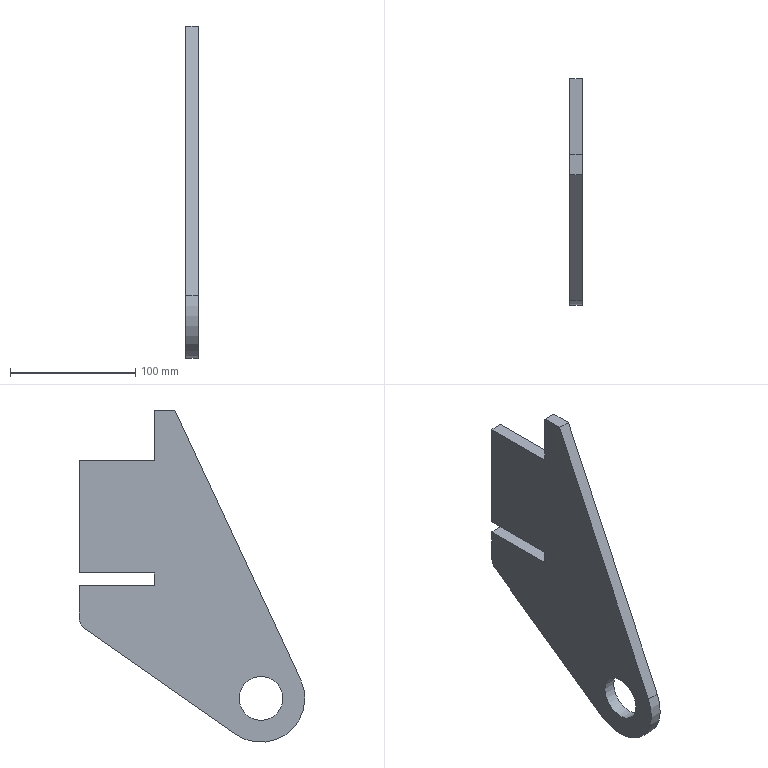Part | STEP file | cylinder mounting plate--000.001--20240927 | 1 solid | 15 faces | box 10 x 180 x 265 mm | volume 256557 mm3 | plane 12 | cylinder 3 | commonest cylinder face diameters 20 x1 35 x1 70 x1
STEP:
#1=CARTESIAN_POINT('',(0.,0.,0.));
#2=DIRECTION('',(0.,0.,1.));
#3=DIRECTION('',(1.,0.,0.));
#4=AXIS2_PLACEMENT_3D('',#1,#2,#3);
#5=CARTESIAN_POINT('',(0.,145.,100.));
#6=VERTEX_POINT('',#5);
#7=CARTESIAN_POINT('',(0.,145.,190.));
#8=VERTEX_POINT('',#7);
#9=CARTESIAN_POINT('',(0.,145.,-567.));
#10=DIRECTION('',(0.,0.,1.));
#11=VECTOR('',#10,1.);
#12=LINE('',#9,#11);
#13=CARTESIAN_POINT('',(1830.173,145.,190.));
#14=DIRECTION('',(0.,-1.,0.));
#15=DIRECTION('',(1.,0.,0.));
#16=AXIS2_PLACEMENT_3D('',#13,#14,#15);
#17=PLANE('',#16);
#18=CARTESIAN_POINT('',(-1830.173,-757.));
#19=DIRECTION('',(0.,1.));
#20=VECTOR('',#19,1.);
#21=LINE('',#18,#20);
#22=(GEOMETRIC_REPRESENTATION_CONTEXT(2)PARAMETRIC_REPRESENTATION_CONTEXT()REPRESENTATION_CONTEXT('',''));
#23=DEFINITIONAL_REPRESENTATION('',(#21),#22);
#24=PCURVE('',#17,#23);
#25=CARTESIAN_POINT('',(0.,145.,-567.));
#26=DIRECTION('',(1.,0.,0.));
#27=DIRECTION('',(0.,1.,0.));
#28=AXIS2_PLACEMENT_3D('',#25,#26,#27);
#29=PLANE('',#28);
#30=CARTESIAN_POINT('',(0.,0.));
#31=DIRECTION('',(0.,1.));
#32=VECTOR('',#31,1.);
#33=LINE('',#30,#32);
#34=(GEOMETRIC_REPRESENTATION_CONTEXT(2)PARAMETRIC_REPRESENTATION_CONTEXT()REPRESENTATION_CONTEXT('',''));
#35=DEFINITIONAL_REPRESENTATION('',(#33),#34);
#36=PCURVE('',#29,#35);
#37=SURFACE_CURVE('',#12,(#24,#36),.PCURVE_S1.);
#38=EDGE_CURVE('',#6,#8,#37,.T.);
#39=ORIENTED_EDGE('',*,*,#38,.F.);
#40=CARTESIAN_POINT('',(-10.,145.,100.));
#41=VERTEX_POINT('',#40);
#42=CARTESIAN_POINT('',(1850.173,145.,100.));
#43=DIRECTION('',(-1.,0.,0.));
#44=VECTOR('',#43,1.);
#45=LINE('',#42,#44);
#46=CARTESIAN_POINT('',(20.,-90.));
#47=DIRECTION('',(-1.,0.));
#48=VECTOR('',#47,1.);
#49=LINE('',#46,#48);
#50=(GEOMETRIC_REPRESENTATION_CONTEXT(2)PARAMETRIC_REPRESENTATION_CONTEXT()REPRESENTATION_CONTEXT('',''));
#51=DEFINITIONAL_REPRESENTATION('',(#49),#50);
#52=PCURVE('',#17,#51);
#53=CARTESIAN_POINT('',(1230.173,85.,100.));
#54=DIRECTION('',(0.,0.,1.));
#55=DIRECTION('',(-0.9613,-0.2756,0.));
#56=AXIS2_PLACEMENT_3D('',#53,#54,#55);
#57=PLANE('',#56);
#58=CARTESIAN_POINT('',(-612.52,113.219));
#59=DIRECTION('',(0.9613,-0.2756));
#60=VECTOR('',#59,1.);
#61=LINE('',#58,#60);
#62=(GEOMETRIC_REPRESENTATION_CONTEXT(2)PARAMETRIC_REPRESENTATION_CONTEXT()REPRESENTATION_CONTEXT('',''));
#63=DEFINITIONAL_REPRESENTATION('',(#61),#62);
#64=PCURVE('',#57,#63);
#65=SURFACE_CURVE('',#45,(#52,#64),.PCURVE_S1.);
#66=EDGE_CURVE('',#6,#41,#65,.T.);
#67=ORIENTED_EDGE('',*,*,#66,.T.);
#68=CARTESIAN_POINT('',(-10.,145.,190.));
#69=VERTEX_POINT('',#68);
#70=CARTESIAN_POINT('',(-10.,145.,-567.));
#71=DIRECTION('',(0.,0.,1.));
#72=VECTOR('',#71,1.);
#73=LINE('',#70,#72);
#74=CARTESIAN_POINT('',(-1840.173,-757.));
#75=DIRECTION('',(0.,1.));
#76=VECTOR('',#75,1.);
#77=LINE('',#74,#76);
#78=(GEOMETRIC_REPRESENTATION_CONTEXT(2)PARAMETRIC_REPRESENTATION_CONTEXT()REPRESENTATION_CONTEXT('',''));
#79=DEFINITIONAL_REPRESENTATION('',(#77),#78);
#80=PCURVE('',#17,#79);
#81=CARTESIAN_POINT('',(-10.,145.,-567.));
#82=DIRECTION('',(1.,0.,0.));
#83=DIRECTION('',(0.,1.,0.));
#84=AXIS2_PLACEMENT_3D('',#81,#82,#83);
#85=PLANE('',#84);
#86=CARTESIAN_POINT('',(0.,0.));
#87=DIRECTION('',(0.,1.));
#88=VECTOR('',#87,1.);
#89=LINE('',#86,#88);
#90=(GEOMETRIC_REPRESENTATION_CONTEXT(2)PARAMETRIC_REPRESENTATION_CONTEXT()REPRESENTATION_CONTEXT('',''));
#91=DEFINITIONAL_REPRESENTATION('',(#89),#90);
#92=PCURVE('',#85,#91);
#93=SURFACE_CURVE('',#73,(#80,#92),.PCURVE_S1.);
#94=EDGE_CURVE('',#41,#69,#93,.T.);
#95=ORIENTED_EDGE('',*,*,#94,.T.);
#96=CARTESIAN_POINT('',(1830.173,145.,190.));
#97=DIRECTION('',(1.,0.,0.));
#98=VECTOR('',#97,1.);
#99=LINE('',#96,#98);
#100=CARTESIAN_POINT('',(0.,0.));
#101=DIRECTION('',(1.,0.));
#102=VECTOR('',#101,1.);
#103=LINE('',#100,#102);
#104=(GEOMETRIC_REPRESENTATION_CONTEXT(2)PARAMETRIC_REPRESENTATION_CONTEXT()REPRESENTATION_CONTEXT('',''));
#105=DEFINITIONAL_REPRESENTATION('',(#103),#104);
#106=PCURVE('',#17,#105);
#107=CARTESIAN_POINT('',(250.,115.,190.));
#108=DIRECTION('',(0.,0.,1.));
#109=DIRECTION('',(-0.2756,0.9613,0.));
#110=AXIS2_PLACEMENT_3D('',#107,#108,#109);
#111=PLANE('',#110);
#112=CARTESIAN_POINT('',(-406.717,-1527.229));
#113=DIRECTION('',(-0.2756,-0.9613));
#114=VECTOR('',#113,1.);
#115=LINE('',#112,#114);
#116=(GEOMETRIC_REPRESENTATION_CONTEXT(2)PARAMETRIC_REPRESENTATION_CONTEXT()REPRESENTATION_CONTEXT('',''));
#117=DEFINITIONAL_REPRESENTATION('',(#115),#116);
#118=PCURVE('',#111,#117);
#119=SURFACE_CURVE('',#99,(#106,#118),.PCURVE_S1.);
#120=EDGE_CURVE('',#69,#8,#119,.T.);
#121=ORIENTED_EDGE('',*,*,#120,.T.);
#122=EDGE_LOOP('',(#39,#67,#95,#121));
#123=FACE_BOUND('',#122,.T.);
#124=ADVANCED_FACE('',(#123),#17,.F.);
#125=CARTESIAN_POINT('',(-10.,-17.5,0.));
#126=VERTEX_POINT('',#125);
#127=CARTESIAN_POINT('',(-10.,0.,0.));
#128=DIRECTION('',(1.,0.,0.));
#129=DIRECTION('',(0.,-1.,0.));
#130=AXIS2_PLACEMENT_3D('',#127,#128,#129);
#131=CIRCLE('',#130,17.5);
#132=CARTESIAN_POINT('',(-145.,567.));
#133=DIRECTION('',(-1.,0.));
#134=AXIS2_PLACEMENT_2D('',#132,#133);
#135=CIRCLE('',#134,17.5);
#136=(GEOMETRIC_REPRESENTATION_CONTEXT(2)PARAMETRIC_REPRESENTATION_CONTEXT()REPRESENTATION_CONTEXT('',''));
#137=DEFINITIONAL_REPRESENTATION('',(#135),#136);
#138=PCURVE('',#85,#137);
#139=CARTESIAN_POINT('',(-360.,0.,0.));
#140=DIRECTION('',(1.,0.,0.));
#141=DIRECTION('',(0.,1.,0.));
#142=AXIS2_PLACEMENT_3D('',#139,#140,#141);
#143=CYLINDRICAL_SURFACE('',#142,17.5);
#144=CARTESIAN_POINT('',(3.142,350.));
#145=DIRECTION('',(1.,0.));
#146=VECTOR('',#145,1.);
#147=LINE('',#144,#146);
#148=(GEOMETRIC_REPRESENTATION_CONTEXT(2)PARAMETRIC_REPRESENTATION_CONTEXT()REPRESENTATION_CONTEXT('',''));
#149=DEFINITIONAL_REPRESENTATION('',(#147),#148);
#150=PCURVE('',#143,#149);
#151=SURFACE_CURVE('',#131,(#138,#150),.PCURVE_S1.);
#152=EDGE_CURVE('',#126,#126,#151,.T.);
#153=ORIENTED_EDGE('',*,*,#152,.T.);
#154=EDGE_LOOP('',(#153));
#155=FACE_BOUND('',#154,.T.);
#156=ORIENTED_EDGE('',*,*,#94,.F.);
#157=CARTESIAN_POINT('',(-10.,85.,100.));
#158=VERTEX_POINT('',#157);
#159=CARTESIAN_POINT('',(-10.,145.,100.));
#160=DIRECTION('',(0.,-1.,0.));
#161=VECTOR('',#160,1.);
#162=LINE('',#159,#161);
#163=CARTESIAN_POINT('',(0.,667.));
#164=DIRECTION('',(-1.,0.));
#165=VECTOR('',#164,1.);
#166=LINE('',#163,#165);
#167=(GEOMETRIC_REPRESENTATION_CONTEXT(2)PARAMETRIC_REPRESENTATION_CONTEXT()REPRESENTATION_CONTEXT('',''));
#168=DEFINITIONAL_REPRESENTATION('',(#166),#167);
#169=PCURVE('',#85,#168);
#170=CARTESIAN_POINT('',(1175.593,-399.514));
#171=DIRECTION('',(0.2756,0.9613));
#172=VECTOR('',#171,1.);
#173=LINE('',#170,#172);
#174=(GEOMETRIC_REPRESENTATION_CONTEXT(2)PARAMETRIC_REPRESENTATION_CONTEXT()REPRESENTATION_CONTEXT('',''));
#175=DEFINITIONAL_REPRESENTATION('',(#173),#174);
#176=PCURVE('',#57,#175);
#177=SURFACE_CURVE('',#162,(#169,#176),.PCURVE_S1.);
#178=EDGE_CURVE('',#41,#158,#177,.T.);
#179=ORIENTED_EDGE('',*,*,#178,.T.);
#180=CARTESIAN_POINT('',(-10.,85.,90.));
#181=VERTEX_POINT('',#180);
#182=CARTESIAN_POINT('',(-10.,85.,-567.));
#183=DIRECTION('',(0.,0.,1.));
#184=VECTOR('',#183,1.);
#185=LINE('',#182,#184);
#186=CARTESIAN_POINT('',(-60.,0.));
#187=DIRECTION('',(0.,1.));
#188=VECTOR('',#187,1.);
#189=LINE('',#186,#188);
#190=(GEOMETRIC_REPRESENTATION_CONTEXT(2)PARAMETRIC_REPRESENTATION_CONTEXT()REPRESENTATION_CONTEXT('',''));
#191=DEFINITIONAL_REPRESENTATION('',(#189),#190);
#192=PCURVE('',#85,#191);
#193=CARTESIAN_POINT('',(-140.,85.,311.5));
#194=DIRECTION('',(0.,-1.,0.));
#195=DIRECTION('',(0.,0.,1.));
#196=AXIS2_PLACEMENT_3D('',#193,#194,#195);
#197=PLANE('',#196);
#198=CARTESIAN_POINT('',(-878.5,-130.));
#199=DIRECTION('',(1.,0.));
#200=VECTOR('',#199,1.);
#201=LINE('',#198,#200);
#202=(GEOMETRIC_REPRESENTATION_CONTEXT(2)PARAMETRIC_REPRESENTATION_CONTEXT()REPRESENTATION_CONTEXT('',''));
#203=DEFINITIONAL_REPRESENTATION('',(#201),#202);
#204=PCURVE('',#197,#203);
#205=SURFACE_CURVE('',#185,(#192,#204),.PCURVE_S1.);
#206=EDGE_CURVE('',#181,#158,#205,.T.);
#207=ORIENTED_EDGE('',*,*,#206,.F.);
#208=CARTESIAN_POINT('',(-10.,145.,90.));
#209=VERTEX_POINT('',#208);
#210=CARTESIAN_POINT('',(-10.,145.,90.));
#211=DIRECTION('',(0.,-1.,0.));
#212=VECTOR('',#211,1.);
#213=LINE('',#210,#212);
#214=CARTESIAN_POINT('',(0.,657.));
#215=DIRECTION('',(-1.,0.));
#216=VECTOR('',#215,1.);
#217=LINE('',#214,#216);
#218=(GEOMETRIC_REPRESENTATION_CONTEXT(2)PARAMETRIC_REPRESENTATION_CONTEXT()REPRESENTATION_CONTEXT('',''));
#219=DEFINITIONAL_REPRESENTATION('',(#217),#218);
#220=PCURVE('',#85,#219);
#221=CARTESIAN_POINT('',(1230.173,85.,90.));
#222=DIRECTION('',(0.,0.,1.));
#223=DIRECTION('',(-0.9613,-0.2756,0.));
#224=AXIS2_PLACEMENT_3D('',#221,#222,#223);
#225=PLANE('',#224);
#226=CARTESIAN_POINT('',(1175.593,-399.514));
#227=DIRECTION('',(0.2756,0.9613));
#228=VECTOR('',#227,1.);
#229=LINE('',#226,#228);
#230=(GEOMETRIC_REPRESENTATION_CONTEXT(2)PARAMETRIC_REPRESENTATION_CONTEXT()REPRESENTATION_CONTEXT('',''));
#231=DEFINITIONAL_REPRESENTATION('',(#229),#230);
#232=PCURVE('',#225,#231);
#233=SURFACE_CURVE('',#213,(#220,#232),.PCURVE_S1.);
#234=EDGE_CURVE('',#209,#181,#233,.T.);
#235=ORIENTED_EDGE('',*,*,#234,.F.);
#236=CARTESIAN_POINT('',(-10.,145.,64.009));
#237=VERTEX_POINT('',#236);
#238=CARTESIAN_POINT('',(-10.,145.,-567.));
#239=DIRECTION('',(0.,0.,1.));
#240=VECTOR('',#239,1.);
#241=LINE('',#238,#240);
#242=CARTESIAN_POINT('',(0.,0.));
#243=DIRECTION('',(0.,1.));
#244=VECTOR('',#243,1.);
#245=LINE('',#242,#244);
#246=(GEOMETRIC_REPRESENTATION_CONTEXT(2)PARAMETRIC_REPRESENTATION_CONTEXT()REPRESENTATION_CONTEXT('',''));
#247=DEFINITIONAL_REPRESENTATION('',(#245),#246);
#248=PCURVE('',#85,#247);
#249=CARTESIAN_POINT('',(1830.173,145.,190.));
#250=DIRECTION('',(0.,-1.,0.));
#251=DIRECTION('',(1.,0.,0.));
#252=AXIS2_PLACEMENT_3D('',#249,#250,#251);
#253=PLANE('',#252);
#254=CARTESIAN_POINT('',(-1840.173,-757.));
#255=DIRECTION('',(0.,1.));
#256=VECTOR('',#255,1.);
#257=LINE('',#254,#256);
#258=(GEOMETRIC_REPRESENTATION_CONTEXT(2)PARAMETRIC_REPRESENTATION_CONTEXT()REPRESENTATION_CONTEXT('',''));
#259=DEFINITIONAL_REPRESENTATION('',(#257),#258);
#260=PCURVE('',#253,#259);
#261=SURFACE_CURVE('',#241,(#248,#260),.PCURVE_S1.);
#262=EDGE_CURVE('',#237,#209,#261,.T.);
#263=ORIENTED_EDGE('',*,*,#262,.F.);
#264=CARTESIAN_POINT('',(-10.,140.736,55.817));
#265=VERTEX_POINT('',#264);
#266=CARTESIAN_POINT('',(-10.,135.,64.009));
#267=DIRECTION('',(-1.,0.,0.));
#268=DIRECTION('',(0.,0.,-1.));
#269=AXIS2_PLACEMENT_3D('',#266,#267,#268);
#270=CIRCLE('',#269,10.);
#271=CARTESIAN_POINT('',(-10.,621.009));
#272=CARTESIAN_POINT('',(-27.321,621.009));
#273=CARTESIAN_POINT('',(-18.66,636.009));
#274=CARTESIAN_POINT('',(-10.,651.009));
#275=CARTESIAN_POINT('',(-1.34,636.009));
#276=CARTESIAN_POINT('',(7.321,621.009));
#277=CARTESIAN_POINT('',(-10.,621.009));
#278=(BOUNDED_CURVE()B_SPLINE_CURVE(2,(#271,#272,#273,#274,#275,#276,#277),.UNSPECIFIED.,.T.,.F.)B_SPLINE_CURVE_WITH_KNOTS((1,2,2,2,2,1),(-2.094,0.,2.094,4.189,6.283,8.378),.UNSPECIFIED.)CURVE()GEOMETRIC_REPRESENTATION_ITEM()RATIONAL_B_SPLINE_CURVE((1.,0.5,1.,0.5,1.,0.5,1.))REPRESENTATION_ITEM(''));
#279=(GEOMETRIC_REPRESENTATION_CONTEXT(2)PARAMETRIC_REPRESENTATION_CONTEXT()REPRESENTATION_CONTEXT('',''));
#280=DEFINITIONAL_REPRESENTATION('',(#278),#279);
#281=PCURVE('',#85,#280);
#282=CARTESIAN_POINT('',(250.,135.,64.009));
#283=DIRECTION('',(-1.,0.,0.));
#284=DIRECTION('',(0.,1.,0.));
#285=AXIS2_PLACEMENT_3D('',#282,#283,#284);
#286=CYLINDRICAL_SURFACE('',#285,10.);
#287=CARTESIAN_POINT('',(-4.712,260.));
#288=DIRECTION('',(1.,0.));
#289=VECTOR('',#288,1.);
#290=LINE('',#287,#289);
#291=(GEOMETRIC_REPRESENTATION_CONTEXT(2)PARAMETRIC_REPRESENTATION_CONTEXT()REPRESENTATION_CONTEXT('',''));
#292=DEFINITIONAL_REPRESENTATION('',(#290),#291);
#293=PCURVE('',#286,#292);
#294=SURFACE_CURVE('',#270,(#281,#293),.PCURVE_S1.);
#295=EDGE_CURVE('',#237,#265,#294,.T.);
#296=ORIENTED_EDGE('',*,*,#295,.T.);
#297=CARTESIAN_POINT('',(-10.,20.075,-28.67));
#298=VERTEX_POINT('',#297);
#299=CARTESIAN_POINT('',(-10.,-149.031,-147.08));
#300=DIRECTION('',(0.,-0.8192,-0.5736));
#301=VECTOR('',#300,1.);
#302=LINE('',#299,#301);
#303=CARTESIAN_POINT('',(-294.031,419.92));
#304=DIRECTION('',(-0.8192,-0.5736));
#305=VECTOR('',#304,1.);
#306=LINE('',#303,#305);
#307=(GEOMETRIC_REPRESENTATION_CONTEXT(2)PARAMETRIC_REPRESENTATION_CONTEXT()REPRESENTATION_CONTEXT('',''));
#308=DEFINITIONAL_REPRESENTATION('',(#306),#307);
#309=PCURVE('',#85,#308);
#310=CARTESIAN_POINT('',(250.,114.278,37.291));
#311=DIRECTION('',(0.,0.5736,-0.8192));
#312=DIRECTION('',(0.2756,-0.7874,-0.5514));
#313=AXIS2_PLACEMENT_3D('',#310,#311,#312);
#314=PLANE('',#313);
#315=CARTESIAN_POINT('',(237.323,338.529));
#316=DIRECTION('',(0.9613,0.2756));
#317=VECTOR('',#316,1.);
#318=LINE('',#315,#317);
#319=(GEOMETRIC_REPRESENTATION_CONTEXT(2)PARAMETRIC_REPRESENTATION_CONTEXT()REPRESENTATION_CONTEXT('',''));
#320=DEFINITIONAL_REPRESENTATION('',(#318),#319);
#321=PCURVE('',#314,#320);
#322=SURFACE_CURVE('',#302,(#309,#321),.PCURVE_S1.);
#323=EDGE_CURVE('',#265,#298,#322,.T.);
#324=ORIENTED_EDGE('',*,*,#323,.T.);
#325=CARTESIAN_POINT('',(-10.,-31.721,14.792));
#326=VERTEX_POINT('',#325);
#327=CARTESIAN_POINT('',(-10.,0.,0.));
#328=DIRECTION('',(-1.,0.,0.));
#329=DIRECTION('',(0.,0.,-1.));
#330=AXIS2_PLACEMENT_3D('',#327,#328,#329);
#331=CIRCLE('',#330,35.);
#332=CARTESIAN_POINT('',(-145.,532.));
#333=CARTESIAN_POINT('',(-205.622,532.));
#334=CARTESIAN_POINT('',(-175.311,584.5));
#335=CARTESIAN_POINT('',(-145.,637.));
#336=CARTESIAN_POINT('',(-114.689,584.5));
#337=CARTESIAN_POINT('',(-84.378,532.));
#338=CARTESIAN_POINT('',(-145.,532.));
#339=(BOUNDED_CURVE()B_SPLINE_CURVE(2,(#332,#333,#334,#335,#336,#337,#338),.UNSPECIFIED.,.T.,.F.)B_SPLINE_CURVE_WITH_KNOTS((1,2,2,2,2,1),(-2.094,0.,2.094,4.189,6.283,8.378),.UNSPECIFIED.)CURVE()GEOMETRIC_REPRESENTATION_ITEM()RATIONAL_B_SPLINE_CURVE((1.,0.5,1.,0.5,1.,0.5,1.))REPRESENTATION_ITEM(''));
#340=(GEOMETRIC_REPRESENTATION_CONTEXT(2)PARAMETRIC_REPRESENTATION_CONTEXT()REPRESENTATION_CONTEXT('',''));
#341=DEFINITIONAL_REPRESENTATION('',(#339),#340);
#342=PCURVE('',#85,#341);
#343=CARTESIAN_POINT('',(-30.,0.,0.));
#344=DIRECTION('',(1.,0.,0.));
#345=DIRECTION('',(0.,0.,1.));
#346=AXIS2_PLACEMENT_3D('',#343,#344,#345);
#347=CYLINDRICAL_SURFACE('',#346,35.);
#348=CARTESIAN_POINT('',(9.425,20.));
#349=DIRECTION('',(-1.,0.));
#350=VECTOR('',#349,1.);
#351=LINE('',#348,#350);
#352=(GEOMETRIC_REPRESENTATION_CONTEXT(2)PARAMETRIC_REPRESENTATION_CONTEXT()REPRESENTATION_CONTEXT('',''));
#353=DEFINITIONAL_REPRESENTATION('',(#351),#352);
#354=PCURVE('',#347,#353);
#355=SURFACE_CURVE('',#331,(#342,#354),.PCURVE_S1.);
#356=EDGE_CURVE('',#298,#326,#355,.T.);
#357=ORIENTED_EDGE('',*,*,#356,.T.);
#358=CARTESIAN_POINT('',(-10.,68.633,230.));
#359=VERTEX_POINT('',#358);
#360=CARTESIAN_POINT('',(-10.,-29.629,19.278));
#361=DIRECTION('',(0.,0.4226,0.9063));
#362=VECTOR('',#361,1.);
#363=LINE('',#360,#362);
#364=CARTESIAN_POINT('',(-174.629,586.278));
#365=DIRECTION('',(0.4226,0.9063));
#366=VECTOR('',#365,1.);
#367=LINE('',#364,#366);
#368=(GEOMETRIC_REPRESENTATION_CONTEXT(2)PARAMETRIC_REPRESENTATION_CONTEXT()REPRESENTATION_CONTEXT('',''));
#369=DEFINITIONAL_REPRESENTATION('',(#367),#368);
#370=PCURVE('',#85,#369);
#371=CARTESIAN_POINT('',(-30.,-29.629,19.278));
#372=DIRECTION('',(0.,-0.9063,0.4226));
#373=DIRECTION('',(-1.,0.,0.));
#374=AXIS2_PLACEMENT_3D('',#371,#372,#373);
#375=PLANE('',#374);
#376=CARTESIAN_POINT('',(-20.,0.));
#377=DIRECTION('',(0.,-1.));
#378=VECTOR('',#377,1.);
#379=LINE('',#376,#378);
#380=(GEOMETRIC_REPRESENTATION_CONTEXT(2)PARAMETRIC_REPRESENTATION_CONTEXT()REPRESENTATION_CONTEXT('',''));
#381=DEFINITIONAL_REPRESENTATION('',(#379),#380);
#382=PCURVE('',#375,#381);
#383=SURFACE_CURVE('',#363,(#370,#382),.PCURVE_S1.);
#384=EDGE_CURVE('',#326,#359,#383,.T.);
#385=ORIENTED_EDGE('',*,*,#384,.T.);
#386=CARTESIAN_POINT('',(-10.,85.,230.));
#387=VERTEX_POINT('',#386);
#388=CARTESIAN_POINT('',(-10.,125.,230.));
#389=DIRECTION('',(0.,1.,0.));
#390=VECTOR('',#389,1.);
#391=LINE('',#388,#390);
#392=CARTESIAN_POINT('',(-20.,797.));
#393=DIRECTION('',(1.,0.));
#394=VECTOR('',#393,1.);
#395=LINE('',#392,#394);
#396=(GEOMETRIC_REPRESENTATION_CONTEXT(2)PARAMETRIC_REPRESENTATION_CONTEXT()REPRESENTATION_CONTEXT('',''));
#397=DEFINITIONAL_REPRESENTATION('',(#395),#396);
#398=PCURVE('',#85,#397);
#399=CARTESIAN_POINT('',(1250.173,125.,230.));
#400=DIRECTION('',(0.,0.,-1.));
#401=DIRECTION('',(0.9613,0.2756,0.));
#402=AXIS2_PLACEMENT_3D('',#399,#400,#401);
#403=PLANE('',#402);
#404=CARTESIAN_POINT('',(-1211.356,-347.351));
#405=DIRECTION('',(0.2756,-0.9613));
#406=VECTOR('',#405,1.);
#407=LINE('',#404,#406);
#408=(GEOMETRIC_REPRESENTATION_CONTEXT(2)PARAMETRIC_REPRESENTATION_CONTEXT()REPRESENTATION_CONTEXT('',''));
#409=DEFINITIONAL_REPRESENTATION('',(#407),#408);
#410=PCURVE('',#403,#409);
#411=SURFACE_CURVE('',#391,(#398,#410),.PCURVE_S1.);
#412=EDGE_CURVE('',#359,#387,#411,.T.);
#413=ORIENTED_EDGE('',*,*,#412,.T.);
#414=CARTESIAN_POINT('',(-10.,85.,190.));
#415=VERTEX_POINT('',#414);
#416=CARTESIAN_POINT('',(-10.,85.,150.));
#417=DIRECTION('',(0.,0.,1.));
#418=VECTOR('',#417,1.);
#419=LINE('',#416,#418);
#420=CARTESIAN_POINT('',(-60.,717.));
#421=DIRECTION('',(0.,1.));
#422=VECTOR('',#421,1.);
#423=LINE('',#420,#422);
#424=(GEOMETRIC_REPRESENTATION_CONTEXT(2)PARAMETRIC_REPRESENTATION_CONTEXT()REPRESENTATION_CONTEXT('',''));
#425=DEFINITIONAL_REPRESENTATION('',(#423),#424);
#426=PCURVE('',#85,#425);
#427=CARTESIAN_POINT('',(-29.759,85.,150.));
#428=DIRECTION('',(0.,1.,0.));
#429=DIRECTION('',(-1.,0.,0.));
#430=AXIS2_PLACEMENT_3D('',#427,#428,#429);
#431=PLANE('',#430);
#432=CARTESIAN_POINT('',(-19.759,0.));
#433=DIRECTION('',(0.,1.));
#434=VECTOR('',#433,1.);
#435=LINE('',#432,#434);
#436=(GEOMETRIC_REPRESENTATION_CONTEXT(2)PARAMETRIC_REPRESENTATION_CONTEXT()REPRESENTATION_CONTEXT('',''));
#437=DEFINITIONAL_REPRESENTATION('',(#435),#436);
#438=PCURVE('',#431,#437);
#439=SURFACE_CURVE('',#419,(#426,#438),.PCURVE_S1.);
#440=EDGE_CURVE('',#415,#387,#439,.T.);
#441=ORIENTED_EDGE('',*,*,#440,.F.);
#442=CARTESIAN_POINT('',(-10.,145.,190.));
#443=DIRECTION('',(0.,-1.,0.));
#444=VECTOR('',#443,1.);
#445=LINE('',#442,#444);
#446=CARTESIAN_POINT('',(0.,757.));
#447=DIRECTION('',(-1.,0.));
#448=VECTOR('',#447,1.);
#449=LINE('',#446,#448);
#450=(GEOMETRIC_REPRESENTATION_CONTEXT(2)PARAMETRIC_REPRESENTATION_CONTEXT()REPRESENTATION_CONTEXT('',''));
#451=DEFINITIONAL_REPRESENTATION('',(#449),#450);
#452=PCURVE('',#85,#451);
#453=CARTESIAN_POINT('',(100.504,241.659));
#454=DIRECTION('',(-0.9613,0.2756));
#455=VECTOR('',#454,1.);
#456=LINE('',#453,#455);
#457=(GEOMETRIC_REPRESENTATION_CONTEXT(2)PARAMETRIC_REPRESENTATION_CONTEXT()REPRESENTATION_CONTEXT('',''));
#458=DEFINITIONAL_REPRESENTATION('',(#456),#457);
#459=PCURVE('',#111,#458);
#460=SURFACE_CURVE('',#445,(#452,#459),.PCURVE_S1.);
#461=EDGE_CURVE('',#69,#415,#460,.T.);
#462=ORIENTED_EDGE('',*,*,#461,.F.);
#463=EDGE_LOOP('',(#156,#179,#207,#235,#263,#296,#324,#357,#385,#413,#441,#462));
#464=FACE_BOUND('',#463,.T.);
#465=ADVANCED_FACE('',(#155,#464),#85,.F.);
#466=CARTESIAN_POINT('',(0.,85.,100.));
#467=VERTEX_POINT('',#466);
#468=CARTESIAN_POINT('',(0.,145.,100.));
#469=DIRECTION('',(0.,-1.,0.));
#470=VECTOR('',#469,1.);
#471=LINE('',#468,#470);
#472=CARTESIAN_POINT('',(0.,667.));
#473=DIRECTION('',(-1.,0.));
#474=VECTOR('',#473,1.);
#475=LINE('',#472,#474);
#476=(GEOMETRIC_REPRESENTATION_CONTEXT(2)PARAMETRIC_REPRESENTATION_CONTEXT()REPRESENTATION_CONTEXT('',''));
#477=DEFINITIONAL_REPRESENTATION('',(#475),#476);
#478=PCURVE('',#29,#477);
#479=CARTESIAN_POINT('',(1165.98,-396.757));
#480=DIRECTION('',(0.2756,0.9613));
#481=VECTOR('',#480,1.);
#482=LINE('',#479,#481);
#483=(GEOMETRIC_REPRESENTATION_CONTEXT(2)PARAMETRIC_REPRESENTATION_CONTEXT()REPRESENTATION_CONTEXT('',''));
#484=DEFINITIONAL_REPRESENTATION('',(#482),#483);
#485=PCURVE('',#57,#484);
#486=SURFACE_CURVE('',#471,(#478,#485),.PCURVE_S1.);
#487=EDGE_CURVE('',#6,#467,#486,.T.);
#488=ORIENTED_EDGE('',*,*,#487,.F.);
#489=ORIENTED_EDGE('',*,*,#38,.T.);
#490=CARTESIAN_POINT('',(0.,85.,190.));
#491=VERTEX_POINT('',#490);
#492=CARTESIAN_POINT('',(0.,145.,190.));
#493=DIRECTION('',(0.,-1.,0.));
#494=VECTOR('',#493,1.);
#495=LINE('',#492,#494);
#496=CARTESIAN_POINT('',(0.,757.));
#497=DIRECTION('',(-1.,0.));
#498=VECTOR('',#497,1.);
#499=LINE('',#496,#498);
#500=(GEOMETRIC_REPRESENTATION_CONTEXT(2)PARAMETRIC_REPRESENTATION_CONTEXT()REPRESENTATION_CONTEXT('',''));
#501=DEFINITIONAL_REPRESENTATION('',(#499),#500);
#502=PCURVE('',#29,#501);
#503=CARTESIAN_POINT('',(97.747,232.046));
#504=DIRECTION('',(-0.9613,0.2756));
#505=VECTOR('',#504,1.);
#506=LINE('',#503,#505);
#507=(GEOMETRIC_REPRESENTATION_CONTEXT(2)PARAMETRIC_REPRESENTATION_CONTEXT()REPRESENTATION_CONTEXT('',''));
#508=DEFINITIONAL_REPRESENTATION('',(#506),#507);
#509=PCURVE('',#111,#508);
#510=SURFACE_CURVE('',#495,(#502,#509),.PCURVE_S1.);
#511=EDGE_CURVE('',#8,#491,#510,.T.);
#512=ORIENTED_EDGE('',*,*,#511,.T.);
#513=CARTESIAN_POINT('',(0.,85.,230.));
#514=VERTEX_POINT('',#513);
#515=CARTESIAN_POINT('',(0.,85.,150.));
#516=DIRECTION('',(0.,0.,1.));
#517=VECTOR('',#516,1.);
#518=LINE('',#515,#517);
#519=CARTESIAN_POINT('',(-60.,717.));
#520=DIRECTION('',(0.,1.));
#521=VECTOR('',#520,1.);
#522=LINE('',#519,#521);
#523=(GEOMETRIC_REPRESENTATION_CONTEXT(2)PARAMETRIC_REPRESENTATION_CONTEXT()REPRESENTATION_CONTEXT('',''));
#524=DEFINITIONAL_REPRESENTATION('',(#522),#523);
#525=PCURVE('',#29,#524);
#526=CARTESIAN_POINT('',(-29.759,0.));
#527=DIRECTION('',(0.,1.));
#528=VECTOR('',#527,1.);
#529=LINE('',#526,#528);
#530=(GEOMETRIC_REPRESENTATION_CONTEXT(2)PARAMETRIC_REPRESENTATION_CONTEXT()REPRESENTATION_CONTEXT('',''));
#531=DEFINITIONAL_REPRESENTATION('',(#529),#530);
#532=PCURVE('',#431,#531);
#533=SURFACE_CURVE('',#518,(#525,#532),.PCURVE_S1.);
#534=EDGE_CURVE('',#491,#514,#533,.T.);
#535=ORIENTED_EDGE('',*,*,#534,.T.);
#536=CARTESIAN_POINT('',(0.,68.633,230.));
#537=VERTEX_POINT('',#536);
#538=CARTESIAN_POINT('',(0.,125.,230.));
#539=DIRECTION('',(0.,-1.,0.));
#540=VECTOR('',#539,1.);
#541=LINE('',#538,#540);
#542=CARTESIAN_POINT('',(-20.,797.));
#543=DIRECTION('',(-1.,0.));
#544=VECTOR('',#543,1.);
#545=LINE('',#542,#544);
#546=(GEOMETRIC_REPRESENTATION_CONTEXT(2)PARAMETRIC_REPRESENTATION_CONTEXT()REPRESENTATION_CONTEXT('',''));
#547=DEFINITIONAL_REPRESENTATION('',(#545),#546);
#548=PCURVE('',#29,#547);
#549=CARTESIAN_POINT('',(-1201.744,-344.594));
#550=DIRECTION('',(-0.2756,0.9613));
#551=VECTOR('',#550,1.);
#552=LINE('',#549,#551);
#553=(GEOMETRIC_REPRESENTATION_CONTEXT(2)PARAMETRIC_REPRESENTATION_CONTEXT()REPRESENTATION_CONTEXT('',''));
#554=DEFINITIONAL_REPRESENTATION('',(#552),#553);
#555=PCURVE('',#403,#554);
#556=SURFACE_CURVE('',#541,(#548,#555),.PCURVE_S1.);
#557=EDGE_CURVE('',#514,#537,#556,.T.);
#558=ORIENTED_EDGE('',*,*,#557,.T.);
#559=CARTESIAN_POINT('',(0.,-31.721,14.792));
#560=VERTEX_POINT('',#559);
#561=CARTESIAN_POINT('',(0.,-222.996,-395.4));
#562=DIRECTION('',(0.,-0.4226,-0.9063));
#563=VECTOR('',#562,1.);
#564=LINE('',#561,#563);
#565=CARTESIAN_POINT('',(-367.996,171.6));
#566=DIRECTION('',(-0.4226,-0.9063));
#567=VECTOR('',#566,1.);
#568=LINE('',#565,#567);
#569=(GEOMETRIC_REPRESENTATION_CONTEXT(2)PARAMETRIC_REPRESENTATION_CONTEXT()REPRESENTATION_CONTEXT('',''));
#570=DEFINITIONAL_REPRESENTATION('',(#568),#569);
#571=PCURVE('',#29,#570);
#572=CARTESIAN_POINT('',(-30.,457.547));
#573=DIRECTION('',(0.,1.));
#574=VECTOR('',#573,1.);
#575=LINE('',#572,#574);
#576=(GEOMETRIC_REPRESENTATION_CONTEXT(2)PARAMETRIC_REPRESENTATION_CONTEXT()REPRESENTATION_CONTEXT('',''));
#577=DEFINITIONAL_REPRESENTATION('',(#575),#576);
#578=PCURVE('',#375,#577);
#579=SURFACE_CURVE('',#564,(#571,#578),.PCURVE_S1.);
#580=EDGE_CURVE('',#537,#560,#579,.T.);
#581=ORIENTED_EDGE('',*,*,#580,.T.);
#582=CARTESIAN_POINT('',(0.,20.075,-28.67));
#583=VERTEX_POINT('',#582);
#584=CARTESIAN_POINT('',(0.,0.,0.));
#585=DIRECTION('',(1.,0.,0.));
#586=DIRECTION('',(0.,0.,-1.));
#587=AXIS2_PLACEMENT_3D('',#584,#585,#586);
#588=CIRCLE('',#587,35.);
#589=CARTESIAN_POINT('',(-145.,567.));
#590=DIRECTION('',(0.,-1.));
#591=AXIS2_PLACEMENT_2D('',#589,#590);
#592=CIRCLE('',#591,35.);
#593=(GEOMETRIC_REPRESENTATION_CONTEXT(2)PARAMETRIC_REPRESENTATION_CONTEXT()REPRESENTATION_CONTEXT('',''));
#594=DEFINITIONAL_REPRESENTATION('',(#592),#593);
#595=PCURVE('',#29,#594);
#596=CARTESIAN_POINT('',(-3.142,30.));
#597=DIRECTION('',(1.,0.));
#598=VECTOR('',#597,1.);
#599=LINE('',#596,#598);
#600=(GEOMETRIC_REPRESENTATION_CONTEXT(2)PARAMETRIC_REPRESENTATION_CONTEXT()REPRESENTATION_CONTEXT('',''));
#601=DEFINITIONAL_REPRESENTATION('',(#599),#600);
#602=PCURVE('',#347,#601);
#603=SURFACE_CURVE('',#588,(#595,#602),.PCURVE_S1.);
#604=EDGE_CURVE('',#560,#583,#603,.T.);
#605=ORIENTED_EDGE('',*,*,#604,.T.);
#606=CARTESIAN_POINT('',(0.,140.736,55.817));
#607=VERTEX_POINT('',#606);
#608=CARTESIAN_POINT('',(0.,-149.031,-147.08));
#609=DIRECTION('',(0.,-0.8192,-0.5736));
#610=VECTOR('',#609,1.);
#611=LINE('',#608,#610);
#612=CARTESIAN_POINT('',(-294.031,419.92));
#613=DIRECTION('',(-0.8192,-0.5736));
#614=VECTOR('',#613,1.);
#615=LINE('',#612,#614);
#616=(GEOMETRIC_REPRESENTATION_CONTEXT(2)PARAMETRIC_REPRESENTATION_CONTEXT()REPRESENTATION_CONTEXT('',''));
#617=DEFINITIONAL_REPRESENTATION('',(#615),#616);
#618=PCURVE('',#29,#617);
#619=CARTESIAN_POINT('',(240.079,328.917));
#620=DIRECTION('',(0.9613,0.2756));
#621=VECTOR('',#620,1.);
#622=LINE('',#619,#621);
#623=(GEOMETRIC_REPRESENTATION_CONTEXT(2)PARAMETRIC_REPRESENTATION_CONTEXT()REPRESENTATION_CONTEXT('',''));
#624=DEFINITIONAL_REPRESENTATION('',(#622),#623);
#625=PCURVE('',#314,#624);
#626=SURFACE_CURVE('',#611,(#618,#625),.PCURVE_S1.);
#627=EDGE_CURVE('',#607,#583,#626,.T.);
#628=ORIENTED_EDGE('',*,*,#627,.F.);
#629=CARTESIAN_POINT('',(0.,145.,64.009));
#630=VERTEX_POINT('',#629);
#631=CARTESIAN_POINT('',(0.,135.,64.009));
#632=DIRECTION('',(1.,0.,0.));
#633=DIRECTION('',(0.,0.,-1.));
#634=AXIS2_PLACEMENT_3D('',#631,#632,#633);
#635=CIRCLE('',#634,10.);
#636=CARTESIAN_POINT('',(-10.,631.009));
#637=DIRECTION('',(0.,-1.));
#638=AXIS2_PLACEMENT_2D('',#636,#637);
#639=CIRCLE('',#638,10.);
#640=(GEOMETRIC_REPRESENTATION_CONTEXT(2)PARAMETRIC_REPRESENTATION_CONTEXT()REPRESENTATION_CONTEXT('',''));
#641=DEFINITIONAL_REPRESENTATION('',(#639),#640);
#642=PCURVE('',#29,#641);
#643=CARTESIAN_POINT('',(1.571,250.));
#644=DIRECTION('',(-1.,0.));
#645=VECTOR('',#644,1.);
#646=LINE('',#643,#645);
#647=(GEOMETRIC_REPRESENTATION_CONTEXT(2)PARAMETRIC_REPRESENTATION_CONTEXT()REPRESENTATION_CONTEXT('',''));
#648=DEFINITIONAL_REPRESENTATION('',(#646),#647);
#649=PCURVE('',#286,#648);
#650=SURFACE_CURVE('',#635,(#642,#649),.PCURVE_S1.);
#651=EDGE_CURVE('',#607,#630,#650,.T.);
#652=ORIENTED_EDGE('',*,*,#651,.T.);
#653=CARTESIAN_POINT('',(0.,145.,90.));
#654=VERTEX_POINT('',#653);
#655=CARTESIAN_POINT('',(0.,145.,-567.));
#656=DIRECTION('',(0.,0.,1.));
#657=VECTOR('',#656,1.);
#658=LINE('',#655,#657);
#659=CARTESIAN_POINT('',(0.,0.));
#660=DIRECTION('',(0.,1.));
#661=VECTOR('',#660,1.);
#662=LINE('',#659,#661);
#663=(GEOMETRIC_REPRESENTATION_CONTEXT(2)PARAMETRIC_REPRESENTATION_CONTEXT()REPRESENTATION_CONTEXT('',''));
#664=DEFINITIONAL_REPRESENTATION('',(#662),#663);
#665=PCURVE('',#29,#664);
#666=CARTESIAN_POINT('',(-1830.173,-757.));
#667=DIRECTION('',(0.,1.));
#668=VECTOR('',#667,1.);
#669=LINE('',#666,#668);
#670=(GEOMETRIC_REPRESENTATION_CONTEXT(2)PARAMETRIC_REPRESENTATION_CONTEXT()REPRESENTATION_CONTEXT('',''));
#671=DEFINITIONAL_REPRESENTATION('',(#669),#670);
#672=PCURVE('',#253,#671);
#673=SURFACE_CURVE('',#658,(#665,#672),.PCURVE_S1.);
#674=EDGE_CURVE('',#630,#654,#673,.T.);
#675=ORIENTED_EDGE('',*,*,#674,.T.);
#676=CARTESIAN_POINT('',(0.,85.,90.));
#677=VERTEX_POINT('',#676);
#678=CARTESIAN_POINT('',(0.,145.,90.));
#679=DIRECTION('',(0.,-1.,0.));
#680=VECTOR('',#679,1.);
#681=LINE('',#678,#680);
#682=CARTESIAN_POINT('',(0.,657.));
#683=DIRECTION('',(-1.,0.));
#684=VECTOR('',#683,1.);
#685=LINE('',#682,#684);
#686=(GEOMETRIC_REPRESENTATION_CONTEXT(2)PARAMETRIC_REPRESENTATION_CONTEXT()REPRESENTATION_CONTEXT('',''));
#687=DEFINITIONAL_REPRESENTATION('',(#685),#686);
#688=PCURVE('',#29,#687);
#689=CARTESIAN_POINT('',(1165.98,-396.757));
#690=DIRECTION('',(0.2756,0.9613));
#691=VECTOR('',#690,1.);
#692=LINE('',#689,#691);
#693=(GEOMETRIC_REPRESENTATION_CONTEXT(2)PARAMETRIC_REPRESENTATION_CONTEXT()REPRESENTATION_CONTEXT('',''));
#694=DEFINITIONAL_REPRESENTATION('',(#692),#693);
#695=PCURVE('',#225,#694);
#696=SURFACE_CURVE('',#681,(#688,#695),.PCURVE_S1.);
#697=EDGE_CURVE('',#654,#677,#696,.T.);
#698=ORIENTED_EDGE('',*,*,#697,.T.);
#699=CARTESIAN_POINT('',(0.,85.,-567.));
#700=DIRECTION('',(0.,0.,1.));
#701=VECTOR('',#700,1.);
#702=LINE('',#699,#701);
#703=CARTESIAN_POINT('',(-60.,0.));
#704=DIRECTION('',(0.,1.));
#705=VECTOR('',#704,1.);
#706=LINE('',#703,#705);
#707=(GEOMETRIC_REPRESENTATION_CONTEXT(2)PARAMETRIC_REPRESENTATION_CONTEXT()REPRESENTATION_CONTEXT('',''));
#708=DEFINITIONAL_REPRESENTATION('',(#706),#707);
#709=PCURVE('',#29,#708);
#710=CARTESIAN_POINT('',(-878.5,-140.));
#711=DIRECTION('',(1.,0.));
#712=VECTOR('',#711,1.);
#713=LINE('',#710,#712);
#714=(GEOMETRIC_REPRESENTATION_CONTEXT(2)PARAMETRIC_REPRESENTATION_CONTEXT()REPRESENTATION_CONTEXT('',''));
#715=DEFINITIONAL_REPRESENTATION('',(#713),#714);
#716=PCURVE('',#197,#715);
#717=SURFACE_CURVE('',#702,(#709,#716),.PCURVE_S1.);
#718=EDGE_CURVE('',#677,#467,#717,.T.);
#719=ORIENTED_EDGE('',*,*,#718,.T.);
#720=EDGE_LOOP('',(#488,#489,#512,#535,#558,#581,#605,#628,#652,#675,#698,#719));
#721=FACE_BOUND('',#720,.T.);
#722=CARTESIAN_POINT('',(0.,-17.5,0.));
#723=VERTEX_POINT('',#722);
#724=CARTESIAN_POINT('',(0.,0.,0.));
#725=DIRECTION('',(1.,0.,0.));
#726=DIRECTION('',(0.,-1.,0.));
#727=AXIS2_PLACEMENT_3D('',#724,#725,#726);
#728=CIRCLE('',#727,17.5);
#729=CARTESIAN_POINT('',(-145.,567.));
#730=DIRECTION('',(-1.,0.));
#731=AXIS2_PLACEMENT_2D('',#729,#730);
#732=CIRCLE('',#731,17.5);
#733=(GEOMETRIC_REPRESENTATION_CONTEXT(2)PARAMETRIC_REPRESENTATION_CONTEXT()REPRESENTATION_CONTEXT('',''));
#734=DEFINITIONAL_REPRESENTATION('',(#732),#733);
#735=PCURVE('',#29,#734);
#736=CARTESIAN_POINT('',(3.142,360.));
#737=DIRECTION('',(1.,0.));
#738=VECTOR('',#737,1.);
#739=LINE('',#736,#738);
#740=(GEOMETRIC_REPRESENTATION_CONTEXT(2)PARAMETRIC_REPRESENTATION_CONTEXT()REPRESENTATION_CONTEXT('',''));
#741=DEFINITIONAL_REPRESENTATION('',(#739),#740);
#742=PCURVE('',#143,#741);
#743=SURFACE_CURVE('',#728,(#735,#742),.PCURVE_S1.);
#744=EDGE_CURVE('',#723,#723,#743,.T.);
#745=ORIENTED_EDGE('',*,*,#744,.F.);
#746=EDGE_LOOP('',(#745));
#747=FACE_BOUND('',#746,.T.);
#748=ADVANCED_FACE('',(#721,#747),#29,.T.);
#749=CARTESIAN_POINT('',(1250.173,68.633,230.));
#750=DIRECTION('',(-1.,0.,0.));
#751=VECTOR('',#750,1.);
#752=LINE('',#749,#751);
#753=CARTESIAN_POINT('',(-15.537,54.184));
#754=DIRECTION('',(-0.9613,-0.2756));
#755=VECTOR('',#754,1.);
#756=LINE('',#753,#755);
#757=(GEOMETRIC_REPRESENTATION_CONTEXT(2)PARAMETRIC_REPRESENTATION_CONTEXT()REPRESENTATION_CONTEXT('',''));
#758=DEFINITIONAL_REPRESENTATION('',(#756),#757);
#759=PCURVE('',#403,#758);
#760=CARTESIAN_POINT('',(-1280.173,-232.506));
#761=DIRECTION('',(1.,0.));
#762=VECTOR('',#761,1.);
#763=LINE('',#760,#762);
#764=(GEOMETRIC_REPRESENTATION_CONTEXT(2)PARAMETRIC_REPRESENTATION_CONTEXT()REPRESENTATION_CONTEXT('',''));
#765=DEFINITIONAL_REPRESENTATION('',(#763),#764);
#766=PCURVE('',#375,#765);
#767=SURFACE_CURVE('',#752,(#759,#766),.PCURVE_S1.);
#768=EDGE_CURVE('',#537,#359,#767,.T.);
#769=ORIENTED_EDGE('',*,*,#768,.F.);
#770=ORIENTED_EDGE('',*,*,#557,.F.);
#771=CARTESIAN_POINT('',(-29.759,85.,230.));
#772=DIRECTION('',(-1.,0.,0.));
#773=VECTOR('',#772,1.);
#774=LINE('',#771,#773);
#775=CARTESIAN_POINT('',(-1241.375,-314.347));
#776=DIRECTION('',(-0.9613,-0.2756));
#777=VECTOR('',#776,1.);
#778=LINE('',#775,#777);
#779=(GEOMETRIC_REPRESENTATION_CONTEXT(2)PARAMETRIC_REPRESENTATION_CONTEXT()REPRESENTATION_CONTEXT('',''));
#780=DEFINITIONAL_REPRESENTATION('',(#778),#779);
#781=PCURVE('',#403,#780);
#782=CARTESIAN_POINT('',(0.,80.));
#783=DIRECTION('',(1.,0.));
#784=VECTOR('',#783,1.);
#785=LINE('',#782,#784);
#786=(GEOMETRIC_REPRESENTATION_CONTEXT(2)PARAMETRIC_REPRESENTATION_CONTEXT()REPRESENTATION_CONTEXT('',''));
#787=DEFINITIONAL_REPRESENTATION('',(#785),#786);
#788=PCURVE('',#431,#787);
#789=SURFACE_CURVE('',#774,(#781,#788),.PCURVE_S1.);
#790=EDGE_CURVE('',#514,#387,#789,.T.);
#791=ORIENTED_EDGE('',*,*,#790,.T.);
#792=ORIENTED_EDGE('',*,*,#412,.F.);
#793=EDGE_LOOP('',(#769,#770,#791,#792));
#794=FACE_BOUND('',#793,.T.);
#795=ADVANCED_FACE('',(#794),#403,.F.);
#796=ORIENTED_EDGE('',*,*,#323,.F.);
#797=CARTESIAN_POINT('',(250.,140.736,55.817));
#798=DIRECTION('',(1.,0.,0.));
#799=VECTOR('',#798,1.);
#800=LINE('',#797,#799);
#801=CARTESIAN_POINT('',(-31.048,-8.903));
#802=DIRECTION('',(0.2756,-0.9613));
#803=VECTOR('',#802,1.);
#804=LINE('',#801,#803);
#805=(GEOMETRIC_REPRESENTATION_CONTEXT(2)PARAMETRIC_REPRESENTATION_CONTEXT()REPRESENTATION_CONTEXT('',''));
#806=DEFINITIONAL_REPRESENTATION('',(#804),#805);
#807=PCURVE('',#314,#806);
#808=CARTESIAN_POINT('',(0.9599,0.));
#809=DIRECTION('',(0.,-1.));
#810=VECTOR('',#809,1.);
#811=LINE('',#808,#810);
#812=(GEOMETRIC_REPRESENTATION_CONTEXT(2)PARAMETRIC_REPRESENTATION_CONTEXT()REPRESENTATION_CONTEXT('',''));
#813=DEFINITIONAL_REPRESENTATION('',(#811),#812);
#814=PCURVE('',#286,#813);
#815=SURFACE_CURVE('',#800,(#807,#814),.PCURVE_S1.);
#816=EDGE_CURVE('',#265,#607,#815,.T.);
#817=ORIENTED_EDGE('',*,*,#816,.T.);
#818=ORIENTED_EDGE('',*,*,#627,.T.);
#819=CARTESIAN_POINT('',(250.,20.075,-28.67));
#820=DIRECTION('',(-1.,0.,0.));
#821=VECTOR('',#820,1.);
#822=LINE('',#819,#821);
#823=CARTESIAN_POINT('',(110.545,31.698));
#824=DIRECTION('',(-0.2756,0.9613));
#825=VECTOR('',#824,1.);
#826=LINE('',#823,#825);
#827=(GEOMETRIC_REPRESENTATION_CONTEXT(2)PARAMETRIC_REPRESENTATION_CONTEXT()REPRESENTATION_CONTEXT('',''));
#828=DEFINITIONAL_REPRESENTATION('',(#826),#827);
#829=PCURVE('',#314,#828);
#830=CARTESIAN_POINT('',(3.752,280.));
#831=DIRECTION('',(0.,-1.));
#832=VECTOR('',#831,1.);
#833=LINE('',#830,#832);
#834=(GEOMETRIC_REPRESENTATION_CONTEXT(2)PARAMETRIC_REPRESENTATION_CONTEXT()REPRESENTATION_CONTEXT('',''));
#835=DEFINITIONAL_REPRESENTATION('',(#833),#834);
#836=PCURVE('',#347,#835);
#837=SURFACE_CURVE('',#822,(#829,#836),.PCURVE_S1.);
#838=EDGE_CURVE('',#583,#298,#837,.T.);
#839=ORIENTED_EDGE('',*,*,#838,.T.);
#840=EDGE_LOOP('',(#796,#817,#818,#839));
#841=FACE_BOUND('',#840,.T.);
#842=ADVANCED_FACE('',(#841),#314,.T.);
#843=ORIENTED_EDGE('',*,*,#152,.T.);
#844=CARTESIAN_POINT('',(-10.,-17.5,0.));
#845=CARTESIAN_POINT('',(0.,-17.5,0.));
#846=B_SPLINE_CURVE_WITH_KNOTS('',1,(#844,#845),.UNSPECIFIED.,.F.,.F.,(2,2),(350.,360.),.PIECEWISE_BEZIER_KNOTS.);
#847=CARTESIAN_POINT('',(9.425,0.));
#848=DIRECTION('',(0.,1.));
#849=VECTOR('',#848,1.);
#850=LINE('',#847,#849);
#851=(GEOMETRIC_REPRESENTATION_CONTEXT(2)PARAMETRIC_REPRESENTATION_CONTEXT()REPRESENTATION_CONTEXT('',''));
#852=DEFINITIONAL_REPRESENTATION('',(#850),#851);
#853=PCURVE('',#143,#852);
#854=CARTESIAN_POINT('',(3.142,0.));
#855=DIRECTION('',(0.,1.));
#856=VECTOR('',#855,1.);
#857=LINE('',#854,#856);
#858=(GEOMETRIC_REPRESENTATION_CONTEXT(2)PARAMETRIC_REPRESENTATION_CONTEXT()REPRESENTATION_CONTEXT('',''));
#859=DEFINITIONAL_REPRESENTATION('',(#857),#858);
#860=PCURVE('',#143,#859);
#861=SEAM_CURVE('',#846,(#853,#860),.PCURVE_S1.);
#862=EDGE_CURVE('',#126,#723,#861,.T.);
#863=ORIENTED_EDGE('',*,*,#862,.T.);
#864=ORIENTED_EDGE('',*,*,#744,.F.);
#865=ORIENTED_EDGE('',*,*,#862,.F.);
#866=EDGE_LOOP('',(#843,#863,#864,#865));
#867=FACE_BOUND('',#866,.F.);
#868=ADVANCED_FACE('',(#867),#143,.F.);
#869=CARTESIAN_POINT('',(1850.173,145.,90.));
#870=DIRECTION('',(-1.,0.,0.));
#871=VECTOR('',#870,1.);
#872=LINE('',#869,#871);
#873=CARTESIAN_POINT('',(20.,-100.));
#874=DIRECTION('',(-1.,0.));
#875=VECTOR('',#874,1.);
#876=LINE('',#873,#875);
#877=(GEOMETRIC_REPRESENTATION_CONTEXT(2)PARAMETRIC_REPRESENTATION_CONTEXT()REPRESENTATION_CONTEXT('',''));
#878=DEFINITIONAL_REPRESENTATION('',(#876),#877);
#879=PCURVE('',#253,#878);
#880=CARTESIAN_POINT('',(-612.52,113.219));
#881=DIRECTION('',(0.9613,-0.2756));
#882=VECTOR('',#881,1.);
#883=LINE('',#880,#882);
#884=(GEOMETRIC_REPRESENTATION_CONTEXT(2)PARAMETRIC_REPRESENTATION_CONTEXT()REPRESENTATION_CONTEXT('',''));
#885=DEFINITIONAL_REPRESENTATION('',(#883),#884);
#886=PCURVE('',#225,#885);
#887=SURFACE_CURVE('',#872,(#879,#886),.PCURVE_S1.);
#888=EDGE_CURVE('',#654,#209,#887,.T.);
#889=ORIENTED_EDGE('',*,*,#888,.F.);
#890=ORIENTED_EDGE('',*,*,#674,.F.);
#891=CARTESIAN_POINT('',(1830.173,145.,64.009));
#892=DIRECTION('',(-1.,0.,0.));
#893=VECTOR('',#892,1.);
#894=LINE('',#891,#893);
#895=CARTESIAN_POINT('',(0.,-125.991));
#896=DIRECTION('',(-1.,0.));
#897=VECTOR('',#896,1.);
#898=LINE('',#895,#897);
#899=(GEOMETRIC_REPRESENTATION_CONTEXT(2)PARAMETRIC_REPRESENTATION_CONTEXT()REPRESENTATION_CONTEXT('',''));
#900=DEFINITIONAL_REPRESENTATION('',(#898),#899);
#901=PCURVE('',#253,#900);
#902=CARTESIAN_POINT('',(0.,-1580.173));
#903=DIRECTION('',(0.,1.));
#904=VECTOR('',#903,1.);
#905=LINE('',#902,#904);
#906=(GEOMETRIC_REPRESENTATION_CONTEXT(2)PARAMETRIC_REPRESENTATION_CONTEXT()REPRESENTATION_CONTEXT('',''));
#907=DEFINITIONAL_REPRESENTATION('',(#905),#906);
#908=PCURVE('',#286,#907);
#909=SURFACE_CURVE('',#894,(#901,#908),.PCURVE_S1.);
#910=EDGE_CURVE('',#630,#237,#909,.T.);
#911=ORIENTED_EDGE('',*,*,#910,.T.);
#912=ORIENTED_EDGE('',*,*,#262,.T.);
#913=EDGE_LOOP('',(#889,#890,#911,#912));
#914=FACE_BOUND('',#913,.T.);
#915=ADVANCED_FACE('',(#914),#253,.F.);
#916=CARTESIAN_POINT('',(250.,85.,190.));
#917=DIRECTION('',(1.,0.,0.));
#918=VECTOR('',#917,1.);
#919=LINE('',#916,#918);
#920=CARTESIAN_POINT('',(-28.838,8.269));
#921=DIRECTION('',(-0.2756,-0.9613));
#922=VECTOR('',#921,1.);
#923=LINE('',#920,#922);
#924=(GEOMETRIC_REPRESENTATION_CONTEXT(2)PARAMETRIC_REPRESENTATION_CONTEXT()REPRESENTATION_CONTEXT('',''));
#925=DEFINITIONAL_REPRESENTATION('',(#923),#924);
#926=PCURVE('',#111,#925);
#927=CARTESIAN_POINT('',(-279.759,40.));
#928=DIRECTION('',(-1.,0.));
#929=VECTOR('',#928,1.);
#930=LINE('',#927,#929);
#931=(GEOMETRIC_REPRESENTATION_CONTEXT(2)PARAMETRIC_REPRESENTATION_CONTEXT()REPRESENTATION_CONTEXT('',''));
#932=DEFINITIONAL_REPRESENTATION('',(#930),#931);
#933=PCURVE('',#431,#932);
#934=SURFACE_CURVE('',#919,(#926,#933),.PCURVE_S1.);
#935=EDGE_CURVE('',#415,#491,#934,.T.);
#936=ORIENTED_EDGE('',*,*,#935,.T.);
#937=ORIENTED_EDGE('',*,*,#511,.F.);
#938=ORIENTED_EDGE('',*,*,#120,.F.);
#939=ORIENTED_EDGE('',*,*,#461,.T.);
#940=EDGE_LOOP('',(#936,#937,#938,#939));
#941=FACE_BOUND('',#940,.T.);
#942=ADVANCED_FACE('',(#941),#111,.T.);
#943=ORIENTED_EDGE('',*,*,#384,.F.);
#944=CARTESIAN_POINT('',(-30.,-31.721,14.792));
#945=DIRECTION('',(1.,0.,0.));
#946=VECTOR('',#945,1.);
#947=LINE('',#944,#946);
#948=CARTESIAN_POINT('',(0.,4.95));
#949=DIRECTION('',(-1.,0.));
#950=VECTOR('',#949,1.);
#951=LINE('',#948,#950);
#952=(GEOMETRIC_REPRESENTATION_CONTEXT(2)PARAMETRIC_REPRESENTATION_CONTEXT()REPRESENTATION_CONTEXT('',''));
#953=DEFINITIONAL_REPRESENTATION('',(#951),#952);
#954=PCURVE('',#375,#953);
#955=CARTESIAN_POINT('',(1.134,0.));
#956=DIRECTION('',(0.,1.));
#957=VECTOR('',#956,1.);
#958=LINE('',#955,#957);
#959=(GEOMETRIC_REPRESENTATION_CONTEXT(2)PARAMETRIC_REPRESENTATION_CONTEXT()REPRESENTATION_CONTEXT('',''));
#960=DEFINITIONAL_REPRESENTATION('',(#958),#959);
#961=PCURVE('',#347,#960);
#962=SURFACE_CURVE('',#947,(#954,#961),.PCURVE_S1.);
#963=EDGE_CURVE('',#326,#560,#962,.T.);
#964=ORIENTED_EDGE('',*,*,#963,.T.);
#965=ORIENTED_EDGE('',*,*,#580,.F.);
#966=ORIENTED_EDGE('',*,*,#768,.T.);
#967=EDGE_LOOP('',(#943,#964,#965,#966));
#968=FACE_BOUND('',#967,.T.);
#969=ADVANCED_FACE('',(#968),#375,.T.);
#970=ORIENTED_EDGE('',*,*,#604,.F.);
#971=ORIENTED_EDGE('',*,*,#963,.F.);
#972=ORIENTED_EDGE('',*,*,#356,.F.);
#973=ORIENTED_EDGE('',*,*,#838,.F.);
#974=EDGE_LOOP('',(#970,#971,#972,#973));
#975=FACE_BOUND('',#974,.T.);
#976=ADVANCED_FACE('',(#975),#347,.T.);
#977=ORIENTED_EDGE('',*,*,#651,.F.);
#978=ORIENTED_EDGE('',*,*,#816,.F.);
#979=ORIENTED_EDGE('',*,*,#295,.F.);
#980=ORIENTED_EDGE('',*,*,#910,.F.);
#981=EDGE_LOOP('',(#977,#978,#979,#980));
#982=FACE_BOUND('',#981,.T.);
#983=ADVANCED_FACE('',(#982),#286,.T.);
#984=ORIENTED_EDGE('',*,*,#935,.F.);
#985=ORIENTED_EDGE('',*,*,#440,.T.);
#986=ORIENTED_EDGE('',*,*,#790,.F.);
#987=ORIENTED_EDGE('',*,*,#534,.F.);
#988=EDGE_LOOP('',(#984,#985,#986,#987));
#989=FACE_BOUND('',#988,.T.);
#990=ADVANCED_FACE('',(#989),#431,.T.);
#991=ORIENTED_EDGE('',*,*,#66,.F.);
#992=ORIENTED_EDGE('',*,*,#487,.T.);
#993=CARTESIAN_POINT('',(-140.,85.,100.));
#994=DIRECTION('',(-1.,0.,0.));
#995=VECTOR('',#994,1.);
#996=LINE('',#993,#995);
#997=CARTESIAN_POINT('',(1317.095,-377.671));
#998=DIRECTION('',(0.9613,-0.2756));
#999=VECTOR('',#998,1.);
#1000=LINE('',#997,#999);
#1001=(GEOMETRIC_REPRESENTATION_CONTEXT(2)PARAMETRIC_REPRESENTATION_CONTEXT()REPRESENTATION_CONTEXT('',''));
#1002=DEFINITIONAL_REPRESENTATION('',(#1000),#1001);
#1003=PCURVE('',#57,#1002);
#1004=CARTESIAN_POINT('',(-211.5,0.));
#1005=DIRECTION('',(0.,1.));
#1006=VECTOR('',#1005,1.);
#1007=LINE('',#1004,#1006);
#1008=(GEOMETRIC_REPRESENTATION_CONTEXT(2)PARAMETRIC_REPRESENTATION_CONTEXT()REPRESENTATION_CONTEXT('',''));
#1009=DEFINITIONAL_REPRESENTATION('',(#1007),#1008);
#1010=PCURVE('',#197,#1009);
#1011=SURFACE_CURVE('',#996,(#1003,#1010),.PCURVE_S1.);
#1012=EDGE_CURVE('',#467,#158,#1011,.T.);
#1013=ORIENTED_EDGE('',*,*,#1012,.T.);
#1014=ORIENTED_EDGE('',*,*,#178,.F.);
#1015=EDGE_LOOP('',(#991,#992,#1013,#1014));
#1016=FACE_BOUND('',#1015,.T.);
#1017=ADVANCED_FACE('',(#1016),#57,.F.);
#1018=ORIENTED_EDGE('',*,*,#234,.T.);
#1019=CARTESIAN_POINT('',(-140.,85.,90.));
#1020=DIRECTION('',(-1.,0.,0.));
#1021=VECTOR('',#1020,1.);
#1022=LINE('',#1019,#1021);
#1023=CARTESIAN_POINT('',(1317.095,-377.671));
#1024=DIRECTION('',(0.9613,-0.2756));
#1025=VECTOR('',#1024,1.);
#1026=LINE('',#1023,#1025);
#1027=(GEOMETRIC_REPRESENTATION_CONTEXT(2)PARAMETRIC_REPRESENTATION_CONTEXT()REPRESENTATION_CONTEXT('',''));
#1028=DEFINITIONAL_REPRESENTATION('',(#1026),#1027);
#1029=PCURVE('',#225,#1028);
#1030=CARTESIAN_POINT('',(-221.5,0.));
#1031=DIRECTION('',(0.,1.));
#1032=VECTOR('',#1031,1.);
#1033=LINE('',#1030,#1032);
#1034=(GEOMETRIC_REPRESENTATION_CONTEXT(2)PARAMETRIC_REPRESENTATION_CONTEXT()REPRESENTATION_CONTEXT('',''));
#1035=DEFINITIONAL_REPRESENTATION('',(#1033),#1034);
#1036=PCURVE('',#197,#1035);
#1037=SURFACE_CURVE('',#1022,(#1029,#1036),.PCURVE_S1.);
#1038=EDGE_CURVE('',#677,#181,#1037,.T.);
#1039=ORIENTED_EDGE('',*,*,#1038,.F.);
#1040=ORIENTED_EDGE('',*,*,#697,.F.);
#1041=ORIENTED_EDGE('',*,*,#888,.T.);
#1042=EDGE_LOOP('',(#1018,#1039,#1040,#1041));
#1043=FACE_BOUND('',#1042,.T.);
#1044=ADVANCED_FACE('',(#1043),#225,.T.);
#1045=ORIENTED_EDGE('',*,*,#206,.T.);
#1046=ORIENTED_EDGE('',*,*,#1012,.F.);
#1047=ORIENTED_EDGE('',*,*,#718,.F.);
#1048=ORIENTED_EDGE('',*,*,#1038,.T.);
#1049=EDGE_LOOP('',(#1045,#1046,#1047,#1048));
#1050=FACE_BOUND('',#1049,.T.);
#1051=ADVANCED_FACE('',(#1050),#197,.F.);
#1052=CLOSED_SHELL('',(#124,#465,#748,#795,#842,#868,#915,#942,#969,#976,#983,#990,#1017,#1044,#1051));
#1053=MANIFOLD_SOLID_BREP('',#1052);
#1054=(LENGTH_UNIT()NAMED_UNIT(*)SI_UNIT(.MILLI.,.METRE.));
#1055=UNCERTAINTY_MEASURE_WITH_UNIT(LENGTH_MEASURE(0.0000005),#1054,'','');
#1056=(NAMED_UNIT(*)PLANE_ANGLE_UNIT()SI_UNIT($,.RADIAN.));
#1057=(NAMED_UNIT(*)SI_UNIT($,.STERADIAN.)SOLID_ANGLE_UNIT());
#1058=(GEOMETRIC_REPRESENTATION_CONTEXT(3)GLOBAL_UNCERTAINTY_ASSIGNED_CONTEXT((#1055))GLOBAL_UNIT_ASSIGNED_CONTEXT((#1054,#1056,#1057))REPRESENTATION_CONTEXT('',''));
#1059=ADVANCED_BREP_SHAPE_REPRESENTATION('',(#4,#1053),#1058);